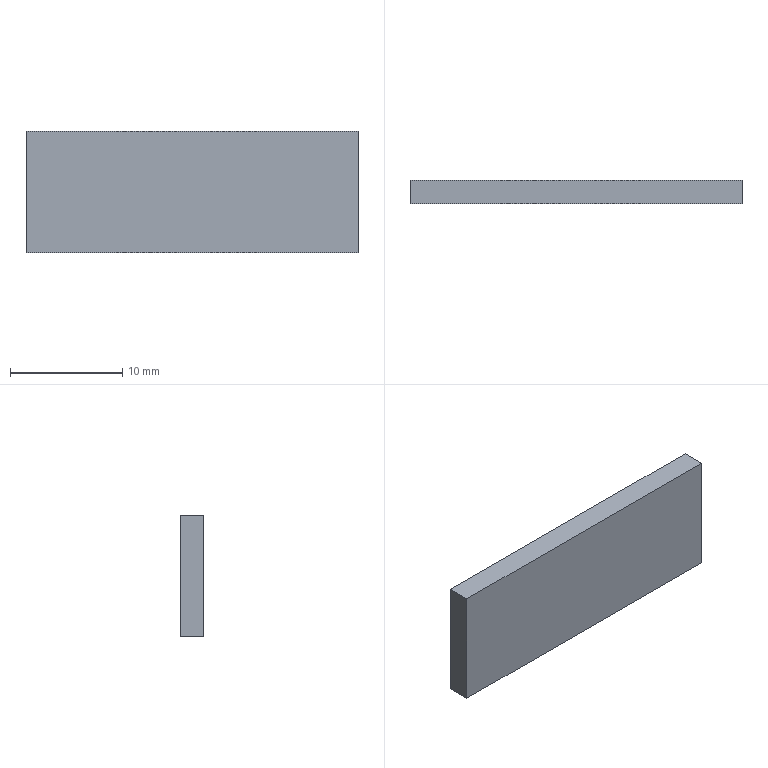Part | STEP file | Part 29.58X10.85X2.08 | 1 solid | 6 faces | box 29.58 x 2.08 x 10.85 mm | volume 667.561 mm3 | plane 6
STEP:
#1=CARTESIAN_POINT('',(0.,0.,0.));
#2=DIRECTION('',(0.,0.,1.));
#3=DIRECTION('',(1.,0.,0.));
#4=AXIS2_PLACEMENT_3D('',#1,#2,#3);
#5=CARTESIAN_POINT('',(14.79,-1.04,5.425));
#6=VERTEX_POINT('',#5);
#7=CARTESIAN_POINT('',(14.79,-1.04,-5.425));
#8=VERTEX_POINT('',#7);
#9=CARTESIAN_POINT('',(14.79,-1.04,-5.425));
#10=DIRECTION('',(0.,0.,-1.));
#11=VECTOR('',#10,1.);
#12=LINE('',#9,#11);
#13=CARTESIAN_POINT('',(14.79,1.04,-5.425));
#14=DIRECTION('',(-1.,0.,0.));
#15=DIRECTION('',(0.,0.,1.));
#16=AXIS2_PLACEMENT_3D('',#13,#14,#15);
#17=PLANE('',#16);
#18=CARTESIAN_POINT('',(0.,-2.08));
#19=DIRECTION('',(-1.,0.));
#20=VECTOR('',#19,1.);
#21=LINE('',#18,#20);
#22=(GEOMETRIC_REPRESENTATION_CONTEXT(2)PARAMETRIC_REPRESENTATION_CONTEXT()REPRESENTATION_CONTEXT('',''));
#23=DEFINITIONAL_REPRESENTATION('',(#21),#22);
#24=PCURVE('',#17,#23);
#25=CARTESIAN_POINT('',(0.,-1.04,0.));
#26=DIRECTION('',(0.,1.,0.));
#27=DIRECTION('',(0.,0.,1.));
#28=AXIS2_PLACEMENT_3D('',#25,#26,#27);
#29=PLANE('',#28);
#30=CARTESIAN_POINT('',(-5.425,14.79));
#31=DIRECTION('',(-1.,0.));
#32=VECTOR('',#31,1.);
#33=LINE('',#30,#32);
#34=(GEOMETRIC_REPRESENTATION_CONTEXT(2)PARAMETRIC_REPRESENTATION_CONTEXT()REPRESENTATION_CONTEXT('',''));
#35=DEFINITIONAL_REPRESENTATION('',(#33),#34);
#36=PCURVE('',#29,#35);
#37=SURFACE_CURVE('',#12,(#24,#36),.PCURVE_S1.);
#38=EDGE_CURVE('',#6,#8,#37,.T.);
#39=ORIENTED_EDGE('',*,*,#38,.T.);
#40=CARTESIAN_POINT('',(14.79,1.04,-5.425));
#41=VERTEX_POINT('',#40);
#42=CARTESIAN_POINT('',(14.79,1.04,-5.425));
#43=DIRECTION('',(0.,-1.,0.));
#44=VECTOR('',#43,1.);
#45=LINE('',#42,#44);
#46=CARTESIAN_POINT('',(0.,0.));
#47=DIRECTION('',(0.,-1.));
#48=VECTOR('',#47,1.);
#49=LINE('',#46,#48);
#50=(GEOMETRIC_REPRESENTATION_CONTEXT(2)PARAMETRIC_REPRESENTATION_CONTEXT()REPRESENTATION_CONTEXT('',''));
#51=DEFINITIONAL_REPRESENTATION('',(#49),#50);
#52=PCURVE('',#17,#51);
#53=CARTESIAN_POINT('',(-14.79,1.04,-5.425));
#54=DIRECTION('',(0.,0.,1.));
#55=DIRECTION('',(1.,0.,0.));
#56=AXIS2_PLACEMENT_3D('',#53,#54,#55);
#57=PLANE('',#56);
#58=CARTESIAN_POINT('',(29.58,0.));
#59=DIRECTION('',(0.,-1.));
#60=VECTOR('',#59,1.);
#61=LINE('',#58,#60);
#62=(GEOMETRIC_REPRESENTATION_CONTEXT(2)PARAMETRIC_REPRESENTATION_CONTEXT()REPRESENTATION_CONTEXT('',''));
#63=DEFINITIONAL_REPRESENTATION('',(#61),#62);
#64=PCURVE('',#57,#63);
#65=SURFACE_CURVE('',#45,(#52,#64),.PCURVE_S1.);
#66=EDGE_CURVE('',#41,#8,#65,.T.);
#67=ORIENTED_EDGE('',*,*,#66,.F.);
#68=CARTESIAN_POINT('',(14.79,1.04,5.425));
#69=VERTEX_POINT('',#68);
#70=CARTESIAN_POINT('',(14.79,1.04,-5.425));
#71=DIRECTION('',(0.,0.,-1.));
#72=VECTOR('',#71,1.);
#73=LINE('',#70,#72);
#74=CARTESIAN_POINT('',(0.,0.));
#75=DIRECTION('',(-1.,0.));
#76=VECTOR('',#75,1.);
#77=LINE('',#74,#76);
#78=(GEOMETRIC_REPRESENTATION_CONTEXT(2)PARAMETRIC_REPRESENTATION_CONTEXT()REPRESENTATION_CONTEXT('',''));
#79=DEFINITIONAL_REPRESENTATION('',(#77),#78);
#80=PCURVE('',#17,#79);
#81=CARTESIAN_POINT('',(0.,1.04,0.));
#82=DIRECTION('',(0.,1.,0.));
#83=DIRECTION('',(0.,0.,1.));
#84=AXIS2_PLACEMENT_3D('',#81,#82,#83);
#85=PLANE('',#84);
#86=CARTESIAN_POINT('',(-5.425,14.79));
#87=DIRECTION('',(-1.,0.));
#88=VECTOR('',#87,1.);
#89=LINE('',#86,#88);
#90=(GEOMETRIC_REPRESENTATION_CONTEXT(2)PARAMETRIC_REPRESENTATION_CONTEXT()REPRESENTATION_CONTEXT('',''));
#91=DEFINITIONAL_REPRESENTATION('',(#89),#90);
#92=PCURVE('',#85,#91);
#93=SURFACE_CURVE('',#73,(#80,#92),.PCURVE_S1.);
#94=EDGE_CURVE('',#69,#41,#93,.T.);
#95=ORIENTED_EDGE('',*,*,#94,.F.);
#96=CARTESIAN_POINT('',(14.79,1.04,5.425));
#97=DIRECTION('',(0.,-1.,0.));
#98=VECTOR('',#97,1.);
#99=LINE('',#96,#98);
#100=CARTESIAN_POINT('',(10.85,0.));
#101=DIRECTION('',(0.,-1.));
#102=VECTOR('',#101,1.);
#103=LINE('',#100,#102);
#104=(GEOMETRIC_REPRESENTATION_CONTEXT(2)PARAMETRIC_REPRESENTATION_CONTEXT()REPRESENTATION_CONTEXT('',''));
#105=DEFINITIONAL_REPRESENTATION('',(#103),#104);
#106=PCURVE('',#17,#105);
#107=CARTESIAN_POINT('',(-14.79,1.04,5.425));
#108=DIRECTION('',(0.,0.,-1.));
#109=DIRECTION('',(-1.,0.,0.));
#110=AXIS2_PLACEMENT_3D('',#107,#108,#109);
#111=PLANE('',#110);
#112=CARTESIAN_POINT('',(-29.58,0.));
#113=DIRECTION('',(0.,-1.));
#114=VECTOR('',#113,1.);
#115=LINE('',#112,#114);
#116=(GEOMETRIC_REPRESENTATION_CONTEXT(2)PARAMETRIC_REPRESENTATION_CONTEXT()REPRESENTATION_CONTEXT('',''));
#117=DEFINITIONAL_REPRESENTATION('',(#115),#116);
#118=PCURVE('',#111,#117);
#119=SURFACE_CURVE('',#99,(#106,#118),.PCURVE_S1.);
#120=EDGE_CURVE('',#69,#6,#119,.T.);
#121=ORIENTED_EDGE('',*,*,#120,.T.);
#122=EDGE_LOOP('',(#39,#67,#95,#121));
#123=FACE_BOUND('',#122,.T.);
#124=ADVANCED_FACE('',(#123),#17,.F.);
#125=CARTESIAN_POINT('',(-14.79,-1.04,-5.425));
#126=VERTEX_POINT('',#125);
#127=CARTESIAN_POINT('',(-14.79,-1.04,-5.425));
#128=DIRECTION('',(-1.,0.,0.));
#129=VECTOR('',#128,1.);
#130=LINE('',#127,#129);
#131=CARTESIAN_POINT('',(0.,-2.08));
#132=DIRECTION('',(-1.,0.));
#133=VECTOR('',#132,1.);
#134=LINE('',#131,#133);
#135=(GEOMETRIC_REPRESENTATION_CONTEXT(2)PARAMETRIC_REPRESENTATION_CONTEXT()REPRESENTATION_CONTEXT('',''));
#136=DEFINITIONAL_REPRESENTATION('',(#134),#135);
#137=PCURVE('',#57,#136);
#138=CARTESIAN_POINT('',(-5.425,-14.79));
#139=DIRECTION('',(0.,-1.));
#140=VECTOR('',#139,1.);
#141=LINE('',#138,#140);
#142=(GEOMETRIC_REPRESENTATION_CONTEXT(2)PARAMETRIC_REPRESENTATION_CONTEXT()REPRESENTATION_CONTEXT('',''));
#143=DEFINITIONAL_REPRESENTATION('',(#141),#142);
#144=PCURVE('',#29,#143);
#145=SURFACE_CURVE('',#130,(#137,#144),.PCURVE_S1.);
#146=EDGE_CURVE('',#8,#126,#145,.T.);
#147=ORIENTED_EDGE('',*,*,#146,.T.);
#148=CARTESIAN_POINT('',(-14.79,1.04,-5.425));
#149=VERTEX_POINT('',#148);
#150=CARTESIAN_POINT('',(-14.79,1.04,-5.425));
#151=DIRECTION('',(0.,-1.,0.));
#152=VECTOR('',#151,1.);
#153=LINE('',#150,#152);
#154=CARTESIAN_POINT('',(0.,0.));
#155=DIRECTION('',(0.,-1.));
#156=VECTOR('',#155,1.);
#157=LINE('',#154,#156);
#158=(GEOMETRIC_REPRESENTATION_CONTEXT(2)PARAMETRIC_REPRESENTATION_CONTEXT()REPRESENTATION_CONTEXT('',''));
#159=DEFINITIONAL_REPRESENTATION('',(#157),#158);
#160=PCURVE('',#57,#159);
#161=CARTESIAN_POINT('',(-14.79,1.04,-5.425));
#162=DIRECTION('',(1.,0.,0.));
#163=DIRECTION('',(0.,0.,-1.));
#164=AXIS2_PLACEMENT_3D('',#161,#162,#163);
#165=PLANE('',#164);
#166=CARTESIAN_POINT('',(0.,0.));
#167=DIRECTION('',(0.,-1.));
#168=VECTOR('',#167,1.);
#169=LINE('',#166,#168);
#170=(GEOMETRIC_REPRESENTATION_CONTEXT(2)PARAMETRIC_REPRESENTATION_CONTEXT()REPRESENTATION_CONTEXT('',''));
#171=DEFINITIONAL_REPRESENTATION('',(#169),#170);
#172=PCURVE('',#165,#171);
#173=SURFACE_CURVE('',#153,(#160,#172),.PCURVE_S1.);
#174=EDGE_CURVE('',#149,#126,#173,.T.);
#175=ORIENTED_EDGE('',*,*,#174,.F.);
#176=CARTESIAN_POINT('',(-14.79,1.04,-5.425));
#177=DIRECTION('',(-1.,0.,0.));
#178=VECTOR('',#177,1.);
#179=LINE('',#176,#178);
#180=CARTESIAN_POINT('',(0.,0.));
#181=DIRECTION('',(-1.,0.));
#182=VECTOR('',#181,1.);
#183=LINE('',#180,#182);
#184=(GEOMETRIC_REPRESENTATION_CONTEXT(2)PARAMETRIC_REPRESENTATION_CONTEXT()REPRESENTATION_CONTEXT('',''));
#185=DEFINITIONAL_REPRESENTATION('',(#183),#184);
#186=PCURVE('',#57,#185);
#187=CARTESIAN_POINT('',(-5.425,-14.79));
#188=DIRECTION('',(0.,-1.));
#189=VECTOR('',#188,1.);
#190=LINE('',#187,#189);
#191=(GEOMETRIC_REPRESENTATION_CONTEXT(2)PARAMETRIC_REPRESENTATION_CONTEXT()REPRESENTATION_CONTEXT('',''));
#192=DEFINITIONAL_REPRESENTATION('',(#190),#191);
#193=PCURVE('',#85,#192);
#194=SURFACE_CURVE('',#179,(#186,#193),.PCURVE_S1.);
#195=EDGE_CURVE('',#41,#149,#194,.T.);
#196=ORIENTED_EDGE('',*,*,#195,.F.);
#197=ORIENTED_EDGE('',*,*,#66,.T.);
#198=EDGE_LOOP('',(#147,#175,#196,#197));
#199=FACE_BOUND('',#198,.T.);
#200=ADVANCED_FACE('',(#199),#57,.F.);
#201=CARTESIAN_POINT('',(-14.79,-1.04,5.425));
#202=VERTEX_POINT('',#201);
#203=CARTESIAN_POINT('',(-14.79,-1.04,-5.425));
#204=DIRECTION('',(0.,0.,1.));
#205=VECTOR('',#204,1.);
#206=LINE('',#203,#205);
#207=CARTESIAN_POINT('',(0.,-2.08));
#208=DIRECTION('',(-1.,0.));
#209=VECTOR('',#208,1.);
#210=LINE('',#207,#209);
#211=(GEOMETRIC_REPRESENTATION_CONTEXT(2)PARAMETRIC_REPRESENTATION_CONTEXT()REPRESENTATION_CONTEXT('',''));
#212=DEFINITIONAL_REPRESENTATION('',(#210),#211);
#213=PCURVE('',#165,#212);
#214=CARTESIAN_POINT('',(-5.425,-14.79));
#215=DIRECTION('',(1.,0.));
#216=VECTOR('',#215,1.);
#217=LINE('',#214,#216);
#218=(GEOMETRIC_REPRESENTATION_CONTEXT(2)PARAMETRIC_REPRESENTATION_CONTEXT()REPRESENTATION_CONTEXT('',''));
#219=DEFINITIONAL_REPRESENTATION('',(#217),#218);
#220=PCURVE('',#29,#219);
#221=SURFACE_CURVE('',#206,(#213,#220),.PCURVE_S1.);
#222=EDGE_CURVE('',#126,#202,#221,.T.);
#223=ORIENTED_EDGE('',*,*,#222,.T.);
#224=CARTESIAN_POINT('',(-14.79,1.04,5.425));
#225=VERTEX_POINT('',#224);
#226=CARTESIAN_POINT('',(-14.79,1.04,5.425));
#227=DIRECTION('',(0.,-1.,0.));
#228=VECTOR('',#227,1.);
#229=LINE('',#226,#228);
#230=CARTESIAN_POINT('',(-10.85,0.));
#231=DIRECTION('',(0.,-1.));
#232=VECTOR('',#231,1.);
#233=LINE('',#230,#232);
#234=(GEOMETRIC_REPRESENTATION_CONTEXT(2)PARAMETRIC_REPRESENTATION_CONTEXT()REPRESENTATION_CONTEXT('',''));
#235=DEFINITIONAL_REPRESENTATION('',(#233),#234);
#236=PCURVE('',#165,#235);
#237=CARTESIAN_POINT('',(0.,0.));
#238=DIRECTION('',(0.,-1.));
#239=VECTOR('',#238,1.);
#240=LINE('',#237,#239);
#241=(GEOMETRIC_REPRESENTATION_CONTEXT(2)PARAMETRIC_REPRESENTATION_CONTEXT()REPRESENTATION_CONTEXT('',''));
#242=DEFINITIONAL_REPRESENTATION('',(#240),#241);
#243=PCURVE('',#111,#242);
#244=SURFACE_CURVE('',#229,(#236,#243),.PCURVE_S1.);
#245=EDGE_CURVE('',#225,#202,#244,.T.);
#246=ORIENTED_EDGE('',*,*,#245,.F.);
#247=CARTESIAN_POINT('',(-14.79,1.04,-5.425));
#248=DIRECTION('',(0.,0.,1.));
#249=VECTOR('',#248,1.);
#250=LINE('',#247,#249);
#251=CARTESIAN_POINT('',(0.,0.));
#252=DIRECTION('',(-1.,0.));
#253=VECTOR('',#252,1.);
#254=LINE('',#251,#253);
#255=(GEOMETRIC_REPRESENTATION_CONTEXT(2)PARAMETRIC_REPRESENTATION_CONTEXT()REPRESENTATION_CONTEXT('',''));
#256=DEFINITIONAL_REPRESENTATION('',(#254),#255);
#257=PCURVE('',#165,#256);
#258=CARTESIAN_POINT('',(-5.425,-14.79));
#259=DIRECTION('',(1.,0.));
#260=VECTOR('',#259,1.);
#261=LINE('',#258,#260);
#262=(GEOMETRIC_REPRESENTATION_CONTEXT(2)PARAMETRIC_REPRESENTATION_CONTEXT()REPRESENTATION_CONTEXT('',''));
#263=DEFINITIONAL_REPRESENTATION('',(#261),#262);
#264=PCURVE('',#85,#263);
#265=SURFACE_CURVE('',#250,(#257,#264),.PCURVE_S1.);
#266=EDGE_CURVE('',#149,#225,#265,.T.);
#267=ORIENTED_EDGE('',*,*,#266,.F.);
#268=ORIENTED_EDGE('',*,*,#174,.T.);
#269=EDGE_LOOP('',(#223,#246,#267,#268));
#270=FACE_BOUND('',#269,.T.);
#271=ADVANCED_FACE('',(#270),#165,.F.);
#272=CARTESIAN_POINT('',(-14.79,-1.04,5.425));
#273=DIRECTION('',(1.,0.,0.));
#274=VECTOR('',#273,1.);
#275=LINE('',#272,#274);
#276=CARTESIAN_POINT('',(0.,-2.08));
#277=DIRECTION('',(-1.,0.));
#278=VECTOR('',#277,1.);
#279=LINE('',#276,#278);
#280=(GEOMETRIC_REPRESENTATION_CONTEXT(2)PARAMETRIC_REPRESENTATION_CONTEXT()REPRESENTATION_CONTEXT('',''));
#281=DEFINITIONAL_REPRESENTATION('',(#279),#280);
#282=PCURVE('',#111,#281);
#283=CARTESIAN_POINT('',(5.425,-14.79));
#284=DIRECTION('',(0.,1.));
#285=VECTOR('',#284,1.);
#286=LINE('',#283,#285);
#287=(GEOMETRIC_REPRESENTATION_CONTEXT(2)PARAMETRIC_REPRESENTATION_CONTEXT()REPRESENTATION_CONTEXT('',''));
#288=DEFINITIONAL_REPRESENTATION('',(#286),#287);
#289=PCURVE('',#29,#288);
#290=SURFACE_CURVE('',#275,(#282,#289),.PCURVE_S1.);
#291=EDGE_CURVE('',#202,#6,#290,.T.);
#292=ORIENTED_EDGE('',*,*,#291,.T.);
#293=ORIENTED_EDGE('',*,*,#120,.F.);
#294=CARTESIAN_POINT('',(-14.79,1.04,5.425));
#295=DIRECTION('',(1.,0.,0.));
#296=VECTOR('',#295,1.);
#297=LINE('',#294,#296);
#298=CARTESIAN_POINT('',(0.,0.));
#299=DIRECTION('',(-1.,0.));
#300=VECTOR('',#299,1.);
#301=LINE('',#298,#300);
#302=(GEOMETRIC_REPRESENTATION_CONTEXT(2)PARAMETRIC_REPRESENTATION_CONTEXT()REPRESENTATION_CONTEXT('',''));
#303=DEFINITIONAL_REPRESENTATION('',(#301),#302);
#304=PCURVE('',#111,#303);
#305=CARTESIAN_POINT('',(5.425,-14.79));
#306=DIRECTION('',(0.,1.));
#307=VECTOR('',#306,1.);
#308=LINE('',#305,#307);
#309=(GEOMETRIC_REPRESENTATION_CONTEXT(2)PARAMETRIC_REPRESENTATION_CONTEXT()REPRESENTATION_CONTEXT('',''));
#310=DEFINITIONAL_REPRESENTATION('',(#308),#309);
#311=PCURVE('',#85,#310);
#312=SURFACE_CURVE('',#297,(#304,#311),.PCURVE_S1.);
#313=EDGE_CURVE('',#225,#69,#312,.T.);
#314=ORIENTED_EDGE('',*,*,#313,.F.);
#315=ORIENTED_EDGE('',*,*,#245,.T.);
#316=EDGE_LOOP('',(#292,#293,#314,#315));
#317=FACE_BOUND('',#316,.T.);
#318=ADVANCED_FACE('',(#317),#111,.F.);
#319=ORIENTED_EDGE('',*,*,#94,.T.);
#320=ORIENTED_EDGE('',*,*,#195,.T.);
#321=ORIENTED_EDGE('',*,*,#266,.T.);
#322=ORIENTED_EDGE('',*,*,#313,.T.);
#323=EDGE_LOOP('',(#319,#320,#321,#322));
#324=FACE_BOUND('',#323,.T.);
#325=ADVANCED_FACE('',(#324),#85,.T.);
#326=ORIENTED_EDGE('',*,*,#38,.F.);
#327=ORIENTED_EDGE('',*,*,#291,.F.);
#328=ORIENTED_EDGE('',*,*,#222,.F.);
#329=ORIENTED_EDGE('',*,*,#146,.F.);
#330=EDGE_LOOP('',(#326,#327,#328,#329));
#331=FACE_BOUND('',#330,.T.);
#332=ADVANCED_FACE('',(#331),#29,.F.);
#333=CLOSED_SHELL('',(#124,#200,#271,#318,#325,#332));
#334=MANIFOLD_SOLID_BREP('',#333);
#335=(LENGTH_UNIT()NAMED_UNIT(*)SI_UNIT(.MILLI.,.METRE.));
#336=UNCERTAINTY_MEASURE_WITH_UNIT(LENGTH_MEASURE(0.0000001),#335,'','');
#337=(NAMED_UNIT(*)PLANE_ANGLE_UNIT()SI_UNIT($,.RADIAN.));
#338=(NAMED_UNIT(*)SI_UNIT($,.STERADIAN.)SOLID_ANGLE_UNIT());
#339=(GEOMETRIC_REPRESENTATION_CONTEXT(3)GLOBAL_UNCERTAINTY_ASSIGNED_CONTEXT((#336))GLOBAL_UNIT_ASSIGNED_CONTEXT((#335,#337,#338))REPRESENTATION_CONTEXT('',''));
#340=ADVANCED_BREP_SHAPE_REPRESENTATION('',(#4,#334),#339);